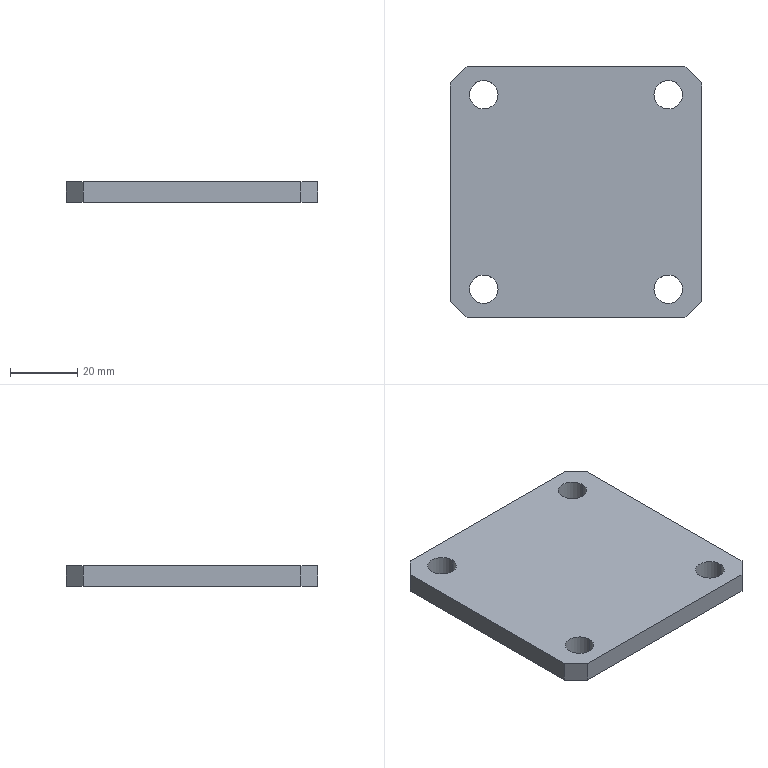Part | SolidWorks | features Extrusion 1 | 1 solid | 18 faces | box 75 x 75 x 6 mm | volume 32088 mm3 | plane 10 | cylinder 8 | commonest cylinder face diameters 8.5 x8
STEP:
#1=CARTESIAN_POINT('',(23.25,-29.,6.));
#2=VERTEX_POINT('',#1);
#3=CARTESIAN_POINT('',(31.75,-29.,6.));
#4=VERTEX_POINT('',#3);
#5=CARTESIAN_POINT('',(27.5,-29.,6.));
#6=DIRECTION('',(0.,0.,1.));
#7=DIRECTION('',(1.,0.,0.));
#8=AXIS2_PLACEMENT_3D('',#5,#6,#7);
#9=CIRCLE('',#8,4.25);
#10=EDGE_CURVE('',#2,#4,#9,.T.);
#11=ORIENTED_EDGE('',*,*,#10,.T.);
#12=CARTESIAN_POINT('',(31.75,-29.,0.));
#13=VERTEX_POINT('',#12);
#14=CARTESIAN_POINT('',(31.75,-29.,6.));
#15=DIRECTION('',(0.,0.,-1.));
#16=VECTOR('',#15,1000.);
#17=LINE('',#14,#16);
#18=EDGE_CURVE('',#4,#13,#17,.T.);
#19=ORIENTED_EDGE('',*,*,#18,.T.);
#20=CARTESIAN_POINT('',(23.25,-29.,0.));
#21=VERTEX_POINT('',#20);
#22=CARTESIAN_POINT('',(27.5,-29.,0.));
#23=DIRECTION('',(0.,0.,1.));
#24=DIRECTION('',(1.,0.,0.));
#25=AXIS2_PLACEMENT_3D('',#22,#23,#24);
#26=CIRCLE('',#25,4.25);
#27=EDGE_CURVE('',#21,#13,#26,.T.);
#28=ORIENTED_EDGE('',*,*,#27,.F.);
#29=CARTESIAN_POINT('',(23.25,-29.,6.));
#30=DIRECTION('',(0.,0.,-1.));
#31=VECTOR('',#30,1000.);
#32=LINE('',#29,#31);
#33=EDGE_CURVE('',#2,#21,#32,.T.);
#34=ORIENTED_EDGE('',*,*,#33,.F.);
#35=EDGE_LOOP('',(#11,#19,#28,#34));
#36=FACE_OUTER_BOUND('',#35,.T.);
#37=CARTESIAN_POINT('',(27.5,-29.,6.));
#38=DIRECTION('',(0.,0.,-1.));
#39=DIRECTION('',(-1.,0.,0.));
#40=AXIS2_PLACEMENT_3D('',#37,#38,#39);
#41=CYLINDRICAL_SURFACE('',#40,4.25);
#42=ADVANCED_FACE('',(#36),#41,.F.);
#43=CARTESIAN_POINT('',(-31.75,-29.,6.));
#44=VERTEX_POINT('',#43);
#45=CARTESIAN_POINT('',(-23.25,-29.,6.));
#46=VERTEX_POINT('',#45);
#47=CARTESIAN_POINT('',(-27.5,-29.,6.));
#48=DIRECTION('',(0.,0.,1.));
#49=DIRECTION('',(1.,0.,0.));
#50=AXIS2_PLACEMENT_3D('',#47,#48,#49);
#51=CIRCLE('',#50,4.25);
#52=EDGE_CURVE('',#44,#46,#51,.T.);
#53=ORIENTED_EDGE('',*,*,#52,.T.);
#54=CARTESIAN_POINT('',(-23.25,-29.,0.));
#55=VERTEX_POINT('',#54);
#56=CARTESIAN_POINT('',(-23.25,-29.,6.));
#57=DIRECTION('',(0.,0.,-1.));
#58=VECTOR('',#57,1000.);
#59=LINE('',#56,#58);
#60=EDGE_CURVE('',#46,#55,#59,.T.);
#61=ORIENTED_EDGE('',*,*,#60,.T.);
#62=CARTESIAN_POINT('',(-31.75,-29.,0.));
#63=VERTEX_POINT('',#62);
#64=CARTESIAN_POINT('',(-27.5,-29.,0.));
#65=DIRECTION('',(0.,0.,1.));
#66=DIRECTION('',(1.,0.,0.));
#67=AXIS2_PLACEMENT_3D('',#64,#65,#66);
#68=CIRCLE('',#67,4.25);
#69=EDGE_CURVE('',#63,#55,#68,.T.);
#70=ORIENTED_EDGE('',*,*,#69,.F.);
#71=CARTESIAN_POINT('',(-31.75,-29.,6.));
#72=DIRECTION('',(0.,0.,-1.));
#73=VECTOR('',#72,1000.);
#74=LINE('',#71,#73);
#75=EDGE_CURVE('',#44,#63,#74,.T.);
#76=ORIENTED_EDGE('',*,*,#75,.F.);
#77=EDGE_LOOP('',(#53,#61,#70,#76));
#78=FACE_OUTER_BOUND('',#77,.T.);
#79=CARTESIAN_POINT('',(-27.5,-29.,6.));
#80=DIRECTION('',(0.,0.,-1.));
#81=DIRECTION('',(-1.,0.,0.));
#82=AXIS2_PLACEMENT_3D('',#79,#80,#81);
#83=CYLINDRICAL_SURFACE('',#82,4.25);
#84=ADVANCED_FACE('',(#78),#83,.F.);
#85=CARTESIAN_POINT('',(23.25,29.,6.));
#86=VERTEX_POINT('',#85);
#87=CARTESIAN_POINT('',(31.75,29.,6.));
#88=VERTEX_POINT('',#87);
#89=CARTESIAN_POINT('',(27.5,29.,6.));
#90=DIRECTION('',(0.,0.,1.));
#91=DIRECTION('',(1.,0.,0.));
#92=AXIS2_PLACEMENT_3D('',#89,#90,#91);
#93=CIRCLE('',#92,4.25);
#94=EDGE_CURVE('',#86,#88,#93,.T.);
#95=ORIENTED_EDGE('',*,*,#94,.T.);
#96=CARTESIAN_POINT('',(31.75,29.,0.));
#97=VERTEX_POINT('',#96);
#98=CARTESIAN_POINT('',(31.75,29.,6.));
#99=DIRECTION('',(0.,0.,-1.));
#100=VECTOR('',#99,1000.);
#101=LINE('',#98,#100);
#102=EDGE_CURVE('',#88,#97,#101,.T.);
#103=ORIENTED_EDGE('',*,*,#102,.T.);
#104=CARTESIAN_POINT('',(23.25,29.,0.));
#105=VERTEX_POINT('',#104);
#106=CARTESIAN_POINT('',(27.5,29.,0.));
#107=DIRECTION('',(0.,0.,1.));
#108=DIRECTION('',(1.,0.,0.));
#109=AXIS2_PLACEMENT_3D('',#106,#107,#108);
#110=CIRCLE('',#109,4.25);
#111=EDGE_CURVE('',#105,#97,#110,.T.);
#112=ORIENTED_EDGE('',*,*,#111,.F.);
#113=CARTESIAN_POINT('',(23.25,29.,6.));
#114=DIRECTION('',(0.,0.,-1.));
#115=VECTOR('',#114,1000.);
#116=LINE('',#113,#115);
#117=EDGE_CURVE('',#86,#105,#116,.T.);
#118=ORIENTED_EDGE('',*,*,#117,.F.);
#119=EDGE_LOOP('',(#95,#103,#112,#118));
#120=FACE_OUTER_BOUND('',#119,.T.);
#121=CARTESIAN_POINT('',(27.5,29.,6.));
#122=DIRECTION('',(0.,0.,-1.));
#123=DIRECTION('',(-1.,0.,0.));
#124=AXIS2_PLACEMENT_3D('',#121,#122,#123);
#125=CYLINDRICAL_SURFACE('',#124,4.25);
#126=ADVANCED_FACE('',(#120),#125,.F.);
#127=CARTESIAN_POINT('',(-31.75,29.,6.));
#128=VERTEX_POINT('',#127);
#129=CARTESIAN_POINT('',(-23.25,29.,6.));
#130=VERTEX_POINT('',#129);
#131=CARTESIAN_POINT('',(-27.5,29.,6.));
#132=DIRECTION('',(0.,0.,1.));
#133=DIRECTION('',(1.,0.,0.));
#134=AXIS2_PLACEMENT_3D('',#131,#132,#133);
#135=CIRCLE('',#134,4.25);
#136=EDGE_CURVE('',#128,#130,#135,.T.);
#137=ORIENTED_EDGE('',*,*,#136,.T.);
#138=CARTESIAN_POINT('',(-23.25,29.,0.));
#139=VERTEX_POINT('',#138);
#140=CARTESIAN_POINT('',(-23.25,29.,6.));
#141=DIRECTION('',(0.,0.,-1.));
#142=VECTOR('',#141,1000.);
#143=LINE('',#140,#142);
#144=EDGE_CURVE('',#130,#139,#143,.T.);
#145=ORIENTED_EDGE('',*,*,#144,.T.);
#146=CARTESIAN_POINT('',(-31.75,29.,0.));
#147=VERTEX_POINT('',#146);
#148=CARTESIAN_POINT('',(-27.5,29.,0.));
#149=DIRECTION('',(0.,0.,1.));
#150=DIRECTION('',(1.,0.,0.));
#151=AXIS2_PLACEMENT_3D('',#148,#149,#150);
#152=CIRCLE('',#151,4.25);
#153=EDGE_CURVE('',#147,#139,#152,.T.);
#154=ORIENTED_EDGE('',*,*,#153,.F.);
#155=CARTESIAN_POINT('',(-31.75,29.,6.));
#156=DIRECTION('',(0.,0.,-1.));
#157=VECTOR('',#156,1000.);
#158=LINE('',#155,#157);
#159=EDGE_CURVE('',#128,#147,#158,.T.);
#160=ORIENTED_EDGE('',*,*,#159,.F.);
#161=EDGE_LOOP('',(#137,#145,#154,#160));
#162=FACE_OUTER_BOUND('',#161,.T.);
#163=CARTESIAN_POINT('',(-27.5,29.,6.));
#164=DIRECTION('',(0.,0.,-1.));
#165=DIRECTION('',(-1.,0.,0.));
#166=AXIS2_PLACEMENT_3D('',#163,#164,#165);
#167=CYLINDRICAL_SURFACE('',#166,4.25);
#168=ADVANCED_FACE('',(#162),#167,.F.);
#169=CARTESIAN_POINT('',(32.5,37.5,6.));
#170=VERTEX_POINT('',#169);
#171=CARTESIAN_POINT('',(-32.5,37.5,6.));
#172=VERTEX_POINT('',#171);
#173=CARTESIAN_POINT('',(-32.5,37.5,6.));
#174=DIRECTION('',(-1.,0.,0.));
#175=VECTOR('',#174,1000.);
#176=LINE('',#173,#175);
#177=EDGE_CURVE('',#170,#172,#176,.T.);
#178=ORIENTED_EDGE('',*,*,#177,.T.);
#179=CARTESIAN_POINT('',(-37.5,32.5,6.));
#180=VERTEX_POINT('',#179);
#181=CARTESIAN_POINT('',(-37.5,32.5,6.));
#182=DIRECTION('',(-0.7071,-0.7071,0.));
#183=VECTOR('',#182,1000.);
#184=LINE('',#181,#183);
#185=EDGE_CURVE('',#172,#180,#184,.T.);
#186=ORIENTED_EDGE('',*,*,#185,.T.);
#187=CARTESIAN_POINT('',(-37.5,-32.5,6.));
#188=VERTEX_POINT('',#187);
#189=CARTESIAN_POINT('',(-37.5,32.5,6.));
#190=DIRECTION('',(0.,-1.,0.));
#191=VECTOR('',#190,1000.);
#192=LINE('',#189,#191);
#193=EDGE_CURVE('',#180,#188,#192,.T.);
#194=ORIENTED_EDGE('',*,*,#193,.T.);
#195=CARTESIAN_POINT('',(-32.5,-37.5,6.));
#196=VERTEX_POINT('',#195);
#197=CARTESIAN_POINT('',(-37.5,-32.5,6.));
#198=DIRECTION('',(0.7071,-0.7071,0.));
#199=VECTOR('',#198,1000.);
#200=LINE('',#197,#199);
#201=EDGE_CURVE('',#188,#196,#200,.T.);
#202=ORIENTED_EDGE('',*,*,#201,.T.);
#203=CARTESIAN_POINT('',(32.5,-37.5,6.));
#204=VERTEX_POINT('',#203);
#205=CARTESIAN_POINT('',(-32.5,-37.5,6.));
#206=DIRECTION('',(1.,0.,0.));
#207=VECTOR('',#206,1000.);
#208=LINE('',#205,#207);
#209=EDGE_CURVE('',#196,#204,#208,.T.);
#210=ORIENTED_EDGE('',*,*,#209,.T.);
#211=CARTESIAN_POINT('',(37.5,-32.5,6.));
#212=VERTEX_POINT('',#211);
#213=CARTESIAN_POINT('',(32.5,-37.5,6.));
#214=DIRECTION('',(0.7071,0.7071,0.));
#215=VECTOR('',#214,1000.);
#216=LINE('',#213,#215);
#217=EDGE_CURVE('',#204,#212,#216,.T.);
#218=ORIENTED_EDGE('',*,*,#217,.T.);
#219=CARTESIAN_POINT('',(37.5,32.5,6.));
#220=VERTEX_POINT('',#219);
#221=CARTESIAN_POINT('',(37.5,32.5,6.));
#222=DIRECTION('',(0.,1.,0.));
#223=VECTOR('',#222,1000.);
#224=LINE('',#221,#223);
#225=EDGE_CURVE('',#212,#220,#224,.T.);
#226=ORIENTED_EDGE('',*,*,#225,.T.);
#227=CARTESIAN_POINT('',(32.5,37.5,6.));
#228=DIRECTION('',(-0.7071,0.7071,0.));
#229=VECTOR('',#228,1000.);
#230=LINE('',#227,#229);
#231=EDGE_CURVE('',#220,#170,#230,.T.);
#232=ORIENTED_EDGE('',*,*,#231,.T.);
#233=EDGE_LOOP('',(#178,#186,#194,#202,#210,#218,#226,#232));
#234=FACE_OUTER_BOUND('',#233,.T.);
#235=ORIENTED_EDGE('',*,*,#136,.F.);
#236=CARTESIAN_POINT('',(-27.5,29.,6.));
#237=DIRECTION('',(0.,0.,1.));
#238=DIRECTION('',(1.,0.,0.));
#239=AXIS2_PLACEMENT_3D('',#236,#237,#238);
#240=CIRCLE('',#239,4.25);
#241=EDGE_CURVE('',#130,#128,#240,.T.);
#242=ORIENTED_EDGE('',*,*,#241,.F.);
#243=EDGE_LOOP('',(#235,#242));
#244=FACE_BOUND('',#243,.T.);
#245=ORIENTED_EDGE('',*,*,#94,.F.);
#246=CARTESIAN_POINT('',(27.5,29.,6.));
#247=DIRECTION('',(0.,0.,1.));
#248=DIRECTION('',(1.,0.,0.));
#249=AXIS2_PLACEMENT_3D('',#246,#247,#248);
#250=CIRCLE('',#249,4.25);
#251=EDGE_CURVE('',#88,#86,#250,.T.);
#252=ORIENTED_EDGE('',*,*,#251,.F.);
#253=EDGE_LOOP('',(#245,#252));
#254=FACE_BOUND('',#253,.T.);
#255=ORIENTED_EDGE('',*,*,#52,.F.);
#256=CARTESIAN_POINT('',(-27.5,-29.,6.));
#257=DIRECTION('',(0.,0.,1.));
#258=DIRECTION('',(1.,0.,0.));
#259=AXIS2_PLACEMENT_3D('',#256,#257,#258);
#260=CIRCLE('',#259,4.25);
#261=EDGE_CURVE('',#46,#44,#260,.T.);
#262=ORIENTED_EDGE('',*,*,#261,.F.);
#263=EDGE_LOOP('',(#255,#262));
#264=FACE_BOUND('',#263,.T.);
#265=ORIENTED_EDGE('',*,*,#10,.F.);
#266=CARTESIAN_POINT('',(27.5,-29.,6.));
#267=DIRECTION('',(0.,0.,1.));
#268=DIRECTION('',(1.,0.,0.));
#269=AXIS2_PLACEMENT_3D('',#266,#267,#268);
#270=CIRCLE('',#269,4.25);
#271=EDGE_CURVE('',#4,#2,#270,.T.);
#272=ORIENTED_EDGE('',*,*,#271,.F.);
#273=EDGE_LOOP('',(#265,#272));
#274=FACE_BOUND('',#273,.T.);
#275=CARTESIAN_POINT('',(0.,0.,6.));
#276=DIRECTION('',(0.,0.,-1.));
#277=DIRECTION('',(-1.,0.,0.));
#278=AXIS2_PLACEMENT_3D('',#275,#276,#277);
#279=PLANE('',#278);
#280=ADVANCED_FACE('',(#234,#244,#254,#264,#274),#279,.F.);
#281=ORIENTED_EDGE('',*,*,#69,.T.);
#282=CARTESIAN_POINT('',(-27.5,-29.,0.));
#283=DIRECTION('',(0.,0.,1.));
#284=DIRECTION('',(1.,0.,0.));
#285=AXIS2_PLACEMENT_3D('',#282,#283,#284);
#286=CIRCLE('',#285,4.25);
#287=EDGE_CURVE('',#55,#63,#286,.T.);
#288=ORIENTED_EDGE('',*,*,#287,.T.);
#289=EDGE_LOOP('',(#281,#288));
#290=FACE_BOUND('',#289,.T.);
#291=ORIENTED_EDGE('',*,*,#153,.T.);
#292=CARTESIAN_POINT('',(-27.5,29.,0.));
#293=DIRECTION('',(0.,0.,1.));
#294=DIRECTION('',(1.,0.,0.));
#295=AXIS2_PLACEMENT_3D('',#292,#293,#294);
#296=CIRCLE('',#295,4.25);
#297=EDGE_CURVE('',#139,#147,#296,.T.);
#298=ORIENTED_EDGE('',*,*,#297,.T.);
#299=EDGE_LOOP('',(#291,#298));
#300=FACE_BOUND('',#299,.T.);
#301=CARTESIAN_POINT('',(32.5,37.5,0.));
#302=VERTEX_POINT('',#301);
#303=CARTESIAN_POINT('',(-32.5,37.5,0.));
#304=VERTEX_POINT('',#303);
#305=CARTESIAN_POINT('',(-32.5,37.5,0.));
#306=DIRECTION('',(-1.,0.,0.));
#307=VECTOR('',#306,1000.);
#308=LINE('',#305,#307);
#309=EDGE_CURVE('',#302,#304,#308,.T.);
#310=ORIENTED_EDGE('',*,*,#309,.F.);
#311=CARTESIAN_POINT('',(37.5,32.5,0.));
#312=VERTEX_POINT('',#311);
#313=CARTESIAN_POINT('',(32.5,37.5,0.));
#314=DIRECTION('',(-0.7071,0.7071,0.));
#315=VECTOR('',#314,1000.);
#316=LINE('',#313,#315);
#317=EDGE_CURVE('',#312,#302,#316,.T.);
#318=ORIENTED_EDGE('',*,*,#317,.F.);
#319=CARTESIAN_POINT('',(37.5,-32.5,0.));
#320=VERTEX_POINT('',#319);
#321=CARTESIAN_POINT('',(37.5,32.5,0.));
#322=DIRECTION('',(0.,1.,0.));
#323=VECTOR('',#322,1000.);
#324=LINE('',#321,#323);
#325=EDGE_CURVE('',#320,#312,#324,.T.);
#326=ORIENTED_EDGE('',*,*,#325,.F.);
#327=CARTESIAN_POINT('',(32.5,-37.5,0.));
#328=VERTEX_POINT('',#327);
#329=CARTESIAN_POINT('',(32.5,-37.5,0.));
#330=DIRECTION('',(0.7071,0.7071,0.));
#331=VECTOR('',#330,1000.);
#332=LINE('',#329,#331);
#333=EDGE_CURVE('',#328,#320,#332,.T.);
#334=ORIENTED_EDGE('',*,*,#333,.F.);
#335=CARTESIAN_POINT('',(-32.5,-37.5,0.));
#336=VERTEX_POINT('',#335);
#337=CARTESIAN_POINT('',(-32.5,-37.5,0.));
#338=DIRECTION('',(1.,0.,0.));
#339=VECTOR('',#338,1000.);
#340=LINE('',#337,#339);
#341=EDGE_CURVE('',#336,#328,#340,.T.);
#342=ORIENTED_EDGE('',*,*,#341,.F.);
#343=CARTESIAN_POINT('',(-37.5,-32.5,0.));
#344=VERTEX_POINT('',#343);
#345=CARTESIAN_POINT('',(-37.5,-32.5,0.));
#346=DIRECTION('',(0.7071,-0.7071,0.));
#347=VECTOR('',#346,1000.);
#348=LINE('',#345,#347);
#349=EDGE_CURVE('',#344,#336,#348,.T.);
#350=ORIENTED_EDGE('',*,*,#349,.F.);
#351=CARTESIAN_POINT('',(-37.5,32.5,0.));
#352=VERTEX_POINT('',#351);
#353=CARTESIAN_POINT('',(-37.5,32.5,0.));
#354=DIRECTION('',(0.,-1.,0.));
#355=VECTOR('',#354,1000.);
#356=LINE('',#353,#355);
#357=EDGE_CURVE('',#352,#344,#356,.T.);
#358=ORIENTED_EDGE('',*,*,#357,.F.);
#359=CARTESIAN_POINT('',(-37.5,32.5,0.));
#360=DIRECTION('',(-0.7071,-0.7071,0.));
#361=VECTOR('',#360,1000.);
#362=LINE('',#359,#361);
#363=EDGE_CURVE('',#304,#352,#362,.T.);
#364=ORIENTED_EDGE('',*,*,#363,.F.);
#365=EDGE_LOOP('',(#310,#318,#326,#334,#342,#350,#358,#364));
#366=FACE_OUTER_BOUND('',#365,.T.);
#367=ORIENTED_EDGE('',*,*,#111,.T.);
#368=CARTESIAN_POINT('',(27.5,29.,0.));
#369=DIRECTION('',(0.,0.,1.));
#370=DIRECTION('',(1.,0.,0.));
#371=AXIS2_PLACEMENT_3D('',#368,#369,#370);
#372=CIRCLE('',#371,4.25);
#373=EDGE_CURVE('',#97,#105,#372,.T.);
#374=ORIENTED_EDGE('',*,*,#373,.T.);
#375=EDGE_LOOP('',(#367,#374));
#376=FACE_BOUND('',#375,.T.);
#377=ORIENTED_EDGE('',*,*,#27,.T.);
#378=CARTESIAN_POINT('',(27.5,-29.,0.));
#379=DIRECTION('',(0.,0.,1.));
#380=DIRECTION('',(1.,0.,0.));
#381=AXIS2_PLACEMENT_3D('',#378,#379,#380);
#382=CIRCLE('',#381,4.25);
#383=EDGE_CURVE('',#13,#21,#382,.T.);
#384=ORIENTED_EDGE('',*,*,#383,.T.);
#385=EDGE_LOOP('',(#377,#384));
#386=FACE_BOUND('',#385,.T.);
#387=CARTESIAN_POINT('',(0.,0.,0.));
#388=DIRECTION('',(0.,0.,-1.));
#389=DIRECTION('',(-1.,0.,0.));
#390=AXIS2_PLACEMENT_3D('',#387,#388,#389);
#391=PLANE('',#390);
#392=ADVANCED_FACE('',(#290,#300,#366,#376,#386),#391,.T.);
#393=ORIENTED_EDGE('',*,*,#309,.T.);
#394=CARTESIAN_POINT('',(-32.5,37.5,6.));
#395=DIRECTION('',(0.,0.,-1.));
#396=VECTOR('',#395,1000.);
#397=LINE('',#394,#396);
#398=EDGE_CURVE('',#172,#304,#397,.T.);
#399=ORIENTED_EDGE('',*,*,#398,.F.);
#400=ORIENTED_EDGE('',*,*,#177,.F.);
#401=CARTESIAN_POINT('',(32.5,37.5,6.));
#402=DIRECTION('',(0.,0.,-1.));
#403=VECTOR('',#402,1000.);
#404=LINE('',#401,#403);
#405=EDGE_CURVE('',#170,#302,#404,.T.);
#406=ORIENTED_EDGE('',*,*,#405,.T.);
#407=EDGE_LOOP('',(#393,#399,#400,#406));
#408=FACE_OUTER_BOUND('',#407,.T.);
#409=CARTESIAN_POINT('',(-32.5,37.5,6.));
#410=DIRECTION('',(0.,-1.,0.));
#411=DIRECTION('',(0.,0.,-1.));
#412=AXIS2_PLACEMENT_3D('',#409,#410,#411);
#413=PLANE('',#412);
#414=ADVANCED_FACE('',(#408),#413,.F.);
#415=ORIENTED_EDGE('',*,*,#363,.T.);
#416=CARTESIAN_POINT('',(-37.5,32.5,6.));
#417=DIRECTION('',(0.,0.,-1.));
#418=VECTOR('',#417,1000.);
#419=LINE('',#416,#418);
#420=EDGE_CURVE('',#180,#352,#419,.T.);
#421=ORIENTED_EDGE('',*,*,#420,.F.);
#422=ORIENTED_EDGE('',*,*,#185,.F.);
#423=ORIENTED_EDGE('',*,*,#398,.T.);
#424=EDGE_LOOP('',(#415,#421,#422,#423));
#425=FACE_OUTER_BOUND('',#424,.T.);
#426=CARTESIAN_POINT('',(-37.5,32.5,6.));
#427=DIRECTION('',(0.7071,-0.7071,0.));
#428=DIRECTION('',(0.7071,0.7071,0.));
#429=AXIS2_PLACEMENT_3D('',#426,#427,#428);
#430=PLANE('',#429);
#431=ADVANCED_FACE('',(#425),#430,.F.);
#432=ORIENTED_EDGE('',*,*,#357,.T.);
#433=CARTESIAN_POINT('',(-37.5,-32.5,6.));
#434=DIRECTION('',(0.,0.,-1.));
#435=VECTOR('',#434,1000.);
#436=LINE('',#433,#435);
#437=EDGE_CURVE('',#188,#344,#436,.T.);
#438=ORIENTED_EDGE('',*,*,#437,.F.);
#439=ORIENTED_EDGE('',*,*,#193,.F.);
#440=ORIENTED_EDGE('',*,*,#420,.T.);
#441=EDGE_LOOP('',(#432,#438,#439,#440));
#442=FACE_OUTER_BOUND('',#441,.T.);
#443=CARTESIAN_POINT('',(-37.5,32.5,6.));
#444=DIRECTION('',(1.,0.,0.));
#445=DIRECTION('',(0.,0.,-1.));
#446=AXIS2_PLACEMENT_3D('',#443,#444,#445);
#447=PLANE('',#446);
#448=ADVANCED_FACE('',(#442),#447,.F.);
#449=ORIENTED_EDGE('',*,*,#349,.T.);
#450=CARTESIAN_POINT('',(-32.5,-37.5,6.));
#451=DIRECTION('',(0.,0.,-1.));
#452=VECTOR('',#451,1000.);
#453=LINE('',#450,#452);
#454=EDGE_CURVE('',#196,#336,#453,.T.);
#455=ORIENTED_EDGE('',*,*,#454,.F.);
#456=ORIENTED_EDGE('',*,*,#201,.F.);
#457=ORIENTED_EDGE('',*,*,#437,.T.);
#458=EDGE_LOOP('',(#449,#455,#456,#457));
#459=FACE_OUTER_BOUND('',#458,.T.);
#460=CARTESIAN_POINT('',(-37.5,-32.5,6.));
#461=DIRECTION('',(0.7071,0.7071,0.));
#462=DIRECTION('',(-0.7071,0.7071,0.));
#463=AXIS2_PLACEMENT_3D('',#460,#461,#462);
#464=PLANE('',#463);
#465=ADVANCED_FACE('',(#459),#464,.F.);
#466=ORIENTED_EDGE('',*,*,#341,.T.);
#467=CARTESIAN_POINT('',(32.5,-37.5,6.));
#468=DIRECTION('',(0.,0.,-1.));
#469=VECTOR('',#468,1000.);
#470=LINE('',#467,#469);
#471=EDGE_CURVE('',#204,#328,#470,.T.);
#472=ORIENTED_EDGE('',*,*,#471,.F.);
#473=ORIENTED_EDGE('',*,*,#209,.F.);
#474=ORIENTED_EDGE('',*,*,#454,.T.);
#475=EDGE_LOOP('',(#466,#472,#473,#474));
#476=FACE_OUTER_BOUND('',#475,.T.);
#477=CARTESIAN_POINT('',(-32.5,-37.5,6.));
#478=DIRECTION('',(0.,1.,0.));
#479=DIRECTION('',(0.,0.,1.));
#480=AXIS2_PLACEMENT_3D('',#477,#478,#479);
#481=PLANE('',#480);
#482=ADVANCED_FACE('',(#476),#481,.F.);
#483=ORIENTED_EDGE('',*,*,#333,.T.);
#484=CARTESIAN_POINT('',(37.5,-32.5,6.));
#485=DIRECTION('',(0.,0.,-1.));
#486=VECTOR('',#485,1000.);
#487=LINE('',#484,#486);
#488=EDGE_CURVE('',#212,#320,#487,.T.);
#489=ORIENTED_EDGE('',*,*,#488,.F.);
#490=ORIENTED_EDGE('',*,*,#217,.F.);
#491=ORIENTED_EDGE('',*,*,#471,.T.);
#492=EDGE_LOOP('',(#483,#489,#490,#491));
#493=FACE_OUTER_BOUND('',#492,.T.);
#494=CARTESIAN_POINT('',(32.5,-37.5,6.));
#495=DIRECTION('',(-0.7071,0.7071,0.));
#496=DIRECTION('',(-0.7071,-0.7071,0.));
#497=AXIS2_PLACEMENT_3D('',#494,#495,#496);
#498=PLANE('',#497);
#499=ADVANCED_FACE('',(#493),#498,.F.);
#500=ORIENTED_EDGE('',*,*,#325,.T.);
#501=CARTESIAN_POINT('',(37.5,32.5,6.));
#502=DIRECTION('',(0.,0.,-1.));
#503=VECTOR('',#502,1000.);
#504=LINE('',#501,#503);
#505=EDGE_CURVE('',#220,#312,#504,.T.);
#506=ORIENTED_EDGE('',*,*,#505,.F.);
#507=ORIENTED_EDGE('',*,*,#225,.F.);
#508=ORIENTED_EDGE('',*,*,#488,.T.);
#509=EDGE_LOOP('',(#500,#506,#507,#508));
#510=FACE_OUTER_BOUND('',#509,.T.);
#511=CARTESIAN_POINT('',(37.5,32.5,6.));
#512=DIRECTION('',(-1.,0.,0.));
#513=DIRECTION('',(0.,-1.,0.));
#514=AXIS2_PLACEMENT_3D('',#511,#512,#513);
#515=PLANE('',#514);
#516=ADVANCED_FACE('',(#510),#515,.F.);
#517=ORIENTED_EDGE('',*,*,#317,.T.);
#518=ORIENTED_EDGE('',*,*,#405,.F.);
#519=ORIENTED_EDGE('',*,*,#231,.F.);
#520=ORIENTED_EDGE('',*,*,#505,.T.);
#521=EDGE_LOOP('',(#517,#518,#519,#520));
#522=FACE_OUTER_BOUND('',#521,.T.);
#523=CARTESIAN_POINT('',(32.5,37.5,6.));
#524=DIRECTION('',(-0.7071,-0.7071,0.));
#525=DIRECTION('',(0.7071,-0.7071,0.));
#526=AXIS2_PLACEMENT_3D('',#523,#524,#525);
#527=PLANE('',#526);
#528=ADVANCED_FACE('',(#522),#527,.F.);
#529=ORIENTED_EDGE('',*,*,#144,.F.);
#530=ORIENTED_EDGE('',*,*,#241,.T.);
#531=ORIENTED_EDGE('',*,*,#159,.T.);
#532=ORIENTED_EDGE('',*,*,#297,.F.);
#533=EDGE_LOOP('',(#529,#530,#531,#532));
#534=FACE_OUTER_BOUND('',#533,.T.);
#535=CARTESIAN_POINT('',(-27.5,29.,6.));
#536=DIRECTION('',(0.,0.,-1.));
#537=DIRECTION('',(-1.,0.,0.));
#538=AXIS2_PLACEMENT_3D('',#535,#536,#537);
#539=CYLINDRICAL_SURFACE('',#538,4.25);
#540=ADVANCED_FACE('',(#534),#539,.F.);
#541=ORIENTED_EDGE('',*,*,#102,.F.);
#542=ORIENTED_EDGE('',*,*,#251,.T.);
#543=ORIENTED_EDGE('',*,*,#117,.T.);
#544=ORIENTED_EDGE('',*,*,#373,.F.);
#545=EDGE_LOOP('',(#541,#542,#543,#544));
#546=FACE_OUTER_BOUND('',#545,.T.);
#547=CARTESIAN_POINT('',(27.5,29.,6.));
#548=DIRECTION('',(0.,0.,-1.));
#549=DIRECTION('',(-1.,0.,0.));
#550=AXIS2_PLACEMENT_3D('',#547,#548,#549);
#551=CYLINDRICAL_SURFACE('',#550,4.25);
#552=ADVANCED_FACE('',(#546),#551,.F.);
#553=ORIENTED_EDGE('',*,*,#60,.F.);
#554=ORIENTED_EDGE('',*,*,#261,.T.);
#555=ORIENTED_EDGE('',*,*,#75,.T.);
#556=ORIENTED_EDGE('',*,*,#287,.F.);
#557=EDGE_LOOP('',(#553,#554,#555,#556));
#558=FACE_OUTER_BOUND('',#557,.T.);
#559=CARTESIAN_POINT('',(-27.5,-29.,6.));
#560=DIRECTION('',(0.,0.,-1.));
#561=DIRECTION('',(-1.,0.,0.));
#562=AXIS2_PLACEMENT_3D('',#559,#560,#561);
#563=CYLINDRICAL_SURFACE('',#562,4.25);
#564=ADVANCED_FACE('',(#558),#563,.F.);
#565=ORIENTED_EDGE('',*,*,#18,.F.);
#566=ORIENTED_EDGE('',*,*,#271,.T.);
#567=ORIENTED_EDGE('',*,*,#33,.T.);
#568=ORIENTED_EDGE('',*,*,#383,.F.);
#569=EDGE_LOOP('',(#565,#566,#567,#568));
#570=FACE_OUTER_BOUND('',#569,.T.);
#571=CARTESIAN_POINT('',(27.5,-29.,6.));
#572=DIRECTION('',(0.,0.,-1.));
#573=DIRECTION('',(-1.,0.,0.));
#574=AXIS2_PLACEMENT_3D('',#571,#572,#573);
#575=CYLINDRICAL_SURFACE('',#574,4.25);
#576=ADVANCED_FACE('',(#570),#575,.F.);
#577=CLOSED_SHELL('',(#42,#84,#126,#168,#280,#392,#414,#431,#448,#465,#482,#499,#516,#528,#540,#552,#564,#576));
#578=MANIFOLD_SOLID_BREP('',#577);
#579=CARTESIAN_POINT('',(0.,0.,0.));
#580=DIRECTION('',(0.,0.,1.));
#581=DIRECTION('',(1.,0.,0.));
#582=AXIS2_PLACEMENT_3D('',#579,#580,#581);
#583=(LENGTH_UNIT()NAMED_UNIT(*)SI_UNIT(.MILLI.,.METRE.));
#584=UNCERTAINTY_MEASURE_WITH_UNIT(LENGTH_MEASURE(0.00001),#583,'','');
#585=(NAMED_UNIT(*)PLANE_ANGLE_UNIT()SI_UNIT($,.RADIAN.));
#586=(NAMED_UNIT(*)SI_UNIT($,.STERADIAN.)SOLID_ANGLE_UNIT());
#587=(GEOMETRIC_REPRESENTATION_CONTEXT(3)GLOBAL_UNCERTAINTY_ASSIGNED_CONTEXT((#584))GLOBAL_UNIT_ASSIGNED_CONTEXT((#583,#585,#586))REPRESENTATION_CONTEXT('',''));
#588=ADVANCED_BREP_SHAPE_REPRESENTATION('',(#578,#582),#587);